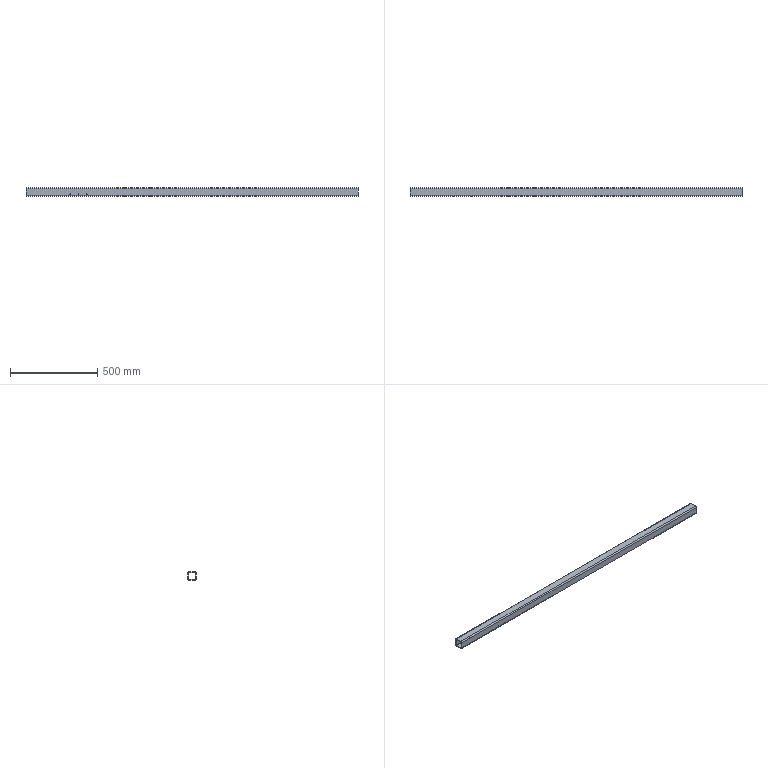Part | NX | 1 solid | 21 faces | box 1900 x 50 x 50 mm | volume 1636478 mm3 | cylinder 11 | plane 10 | commonest cylinder face diameters 4 x4 14 x4 3.3 x3
STEP:
#1=CARTESIAN_POINT('',(-950.,838.,555.));
#2=VERTEX_POINT('',#1);
#3=CARTESIAN_POINT('',(950.,838.,555.));
#4=VERTEX_POINT('',#3);
#5=CARTESIAN_POINT('',(-975.,838.,555.));
#6=DIRECTION('',(1.,0.,0.));
#7=VECTOR('',#6,1000.);
#8=LINE('',#5,#7);
#9=EDGE_CURVE('',#2,#4,#8,.T.);
#10=ORIENTED_EDGE('',*,*,#9,.T.);
#11=CARTESIAN_POINT('',(950.,874.,555.));
#12=VERTEX_POINT('',#11);
#13=CARTESIAN_POINT('',(950.,838.,555.));
#14=DIRECTION('',(0.,1.,0.));
#15=VECTOR('',#14,1000.);
#16=LINE('',#13,#15);
#17=EDGE_CURVE('',#4,#12,#16,.T.);
#18=ORIENTED_EDGE('',*,*,#17,.T.);
#19=CARTESIAN_POINT('',(-950.,874.,555.));
#20=VERTEX_POINT('',#19);
#21=CARTESIAN_POINT('',(-975.,874.,555.));
#22=DIRECTION('',(1.,0.,0.));
#23=VECTOR('',#22,1000.);
#24=LINE('',#21,#23);
#25=EDGE_CURVE('',#20,#12,#24,.T.);
#26=ORIENTED_EDGE('',*,*,#25,.F.);
#27=CARTESIAN_POINT('',(-950.,838.,555.));
#28=DIRECTION('',(0.,-1.,0.));
#29=VECTOR('',#28,1000.);
#30=LINE('',#27,#29);
#31=EDGE_CURVE('',#20,#2,#30,.T.);
#32=ORIENTED_EDGE('',*,*,#31,.T.);
#33=EDGE_LOOP('',(#10,#18,#26,#32));
#34=FACE_BOUND('',#33,.T.);
#35=CARTESIAN_POINT('',(-975.,838.,555.));
#36=DIRECTION('',(0.,0.,1.));
#37=DIRECTION('',(0.,-1.,0.));
#38=AXIS2_PLACEMENT_3D('',#35,#36,#37);
#39=PLANE('',#38);
#40=ADVANCED_FACE('',(#34),#39,.T.);
#41=CARTESIAN_POINT('',(-950.,836.,557.));
#42=VERTEX_POINT('',#41);
#43=CARTESIAN_POINT('',(950.,836.,557.));
#44=VERTEX_POINT('',#43);
#45=CARTESIAN_POINT('',(-975.,836.,557.));
#46=DIRECTION('',(1.,0.,0.));
#47=VECTOR('',#46,1000.);
#48=LINE('',#45,#47);
#49=EDGE_CURVE('',#42,#44,#48,.T.);
#50=ORIENTED_EDGE('',*,*,#49,.T.);
#51=CARTESIAN_POINT('',(950.,838.,557.));
#52=DIRECTION('',(1.,0.,0.));
#53=DIRECTION('',(0.,1.,0.));
#54=AXIS2_PLACEMENT_3D('',#51,#52,#53);
#55=CIRCLE('',#54,2.);
#56=EDGE_CURVE('',#44,#4,#55,.T.);
#57=ORIENTED_EDGE('',*,*,#56,.T.);
#58=ORIENTED_EDGE('',*,*,#9,.F.);
#59=CARTESIAN_POINT('',(-950.,838.,557.));
#60=DIRECTION('',(-1.,0.,0.));
#61=DIRECTION('',(0.,-1.,0.));
#62=AXIS2_PLACEMENT_3D('',#59,#60,#61);
#63=CIRCLE('',#62,2.);
#64=EDGE_CURVE('',#2,#42,#63,.T.);
#65=ORIENTED_EDGE('',*,*,#64,.T.);
#66=EDGE_LOOP('',(#50,#57,#58,#65));
#67=FACE_BOUND('',#66,.T.);
#68=CARTESIAN_POINT('',(-975.,838.,557.));
#69=DIRECTION('',(1.,0.,0.));
#70=DIRECTION('',(0.,0.,-1.));
#71=AXIS2_PLACEMENT_3D('',#68,#69,#70);
#72=CYLINDRICAL_SURFACE('',#71,2.);
#73=ADVANCED_FACE('',(#67),#72,.F.);
#74=CARTESIAN_POINT('',(-650.,836.,560.35));
#75=VERTEX_POINT('',#74);
#76=CARTESIAN_POINT('',(-650.,836.,562.));
#77=DIRECTION('',(0.,-1.,0.));
#78=DIRECTION('',(0.,0.,-1.));
#79=AXIS2_PLACEMENT_3D('',#76,#77,#78);
#80=CIRCLE('',#79,1.65);
#81=EDGE_CURVE('',#75,#75,#80,.T.);
#82=ORIENTED_EDGE('',*,*,#81,.T.);
#83=EDGE_LOOP('',(#82));
#84=FACE_BOUND('',#83,.T.);
#85=CARTESIAN_POINT('',(-602.5,836.,560.35));
#86=VERTEX_POINT('',#85);
#87=CARTESIAN_POINT('',(-602.5,836.,562.));
#88=DIRECTION('',(0.,-1.,0.));
#89=DIRECTION('',(0.,0.,-1.));
#90=AXIS2_PLACEMENT_3D('',#87,#88,#89);
#91=CIRCLE('',#90,1.65);
#92=EDGE_CURVE('',#86,#86,#91,.T.);
#93=ORIENTED_EDGE('',*,*,#92,.T.);
#94=EDGE_LOOP('',(#93));
#95=FACE_BOUND('',#94,.T.);
#96=CARTESIAN_POINT('',(-697.5,836.,560.35));
#97=VERTEX_POINT('',#96);
#98=CARTESIAN_POINT('',(-697.5,836.,562.));
#99=DIRECTION('',(0.,-1.,0.));
#100=DIRECTION('',(0.,0.,-1.));
#101=AXIS2_PLACEMENT_3D('',#98,#99,#100);
#102=CIRCLE('',#101,1.65);
#103=EDGE_CURVE('',#97,#97,#102,.T.);
#104=ORIENTED_EDGE('',*,*,#103,.T.);
#105=EDGE_LOOP('',(#104));
#106=FACE_BOUND('',#105,.T.);
#107=CARTESIAN_POINT('',(-950.,836.,593.));
#108=VERTEX_POINT('',#107);
#109=CARTESIAN_POINT('',(950.,836.,593.));
#110=VERTEX_POINT('',#109);
#111=CARTESIAN_POINT('',(-975.,836.,593.));
#112=DIRECTION('',(1.,0.,0.));
#113=VECTOR('',#112,1000.);
#114=LINE('',#111,#113);
#115=EDGE_CURVE('',#108,#110,#114,.T.);
#116=ORIENTED_EDGE('',*,*,#115,.T.);
#117=CARTESIAN_POINT('',(950.,836.,557.));
#118=DIRECTION('',(0.,0.,-1.));
#119=VECTOR('',#118,1000.);
#120=LINE('',#117,#119);
#121=EDGE_CURVE('',#110,#44,#120,.T.);
#122=ORIENTED_EDGE('',*,*,#121,.T.);
#123=ORIENTED_EDGE('',*,*,#49,.F.);
#124=CARTESIAN_POINT('',(-950.,836.,557.));
#125=DIRECTION('',(0.,0.,1.));
#126=VECTOR('',#125,1000.);
#127=LINE('',#124,#126);
#128=EDGE_CURVE('',#42,#108,#127,.T.);
#129=ORIENTED_EDGE('',*,*,#128,.T.);
#130=EDGE_LOOP('',(#116,#122,#123,#129));
#131=FACE_BOUND('',#130,.T.);
#132=CARTESIAN_POINT('',(-975.,836.,557.));
#133=DIRECTION('',(0.,1.,0.));
#134=DIRECTION('',(0.,0.,1.));
#135=AXIS2_PLACEMENT_3D('',#132,#133,#134);
#136=PLANE('',#135);
#137=ADVANCED_FACE('',(#84,#95,#106,#131),#136,.T.);
#138=CARTESIAN_POINT('',(-950.,838.,595.));
#139=VERTEX_POINT('',#138);
#140=CARTESIAN_POINT('',(950.,838.,595.));
#141=VERTEX_POINT('',#140);
#142=CARTESIAN_POINT('',(-975.,838.,595.));
#143=DIRECTION('',(1.,0.,0.));
#144=VECTOR('',#143,1000.);
#145=LINE('',#142,#144);
#146=EDGE_CURVE('',#139,#141,#145,.T.);
#147=ORIENTED_EDGE('',*,*,#146,.T.);
#148=CARTESIAN_POINT('',(950.,838.,593.));
#149=DIRECTION('',(1.,0.,0.));
#150=DIRECTION('',(0.,1.,0.));
#151=AXIS2_PLACEMENT_3D('',#148,#149,#150);
#152=CIRCLE('',#151,2.);
#153=EDGE_CURVE('',#141,#110,#152,.T.);
#154=ORIENTED_EDGE('',*,*,#153,.T.);
#155=ORIENTED_EDGE('',*,*,#115,.F.);
#156=CARTESIAN_POINT('',(-950.,838.,593.));
#157=DIRECTION('',(-1.,0.,0.));
#158=DIRECTION('',(0.,-1.,0.));
#159=AXIS2_PLACEMENT_3D('',#156,#157,#158);
#160=CIRCLE('',#159,2.);
#161=EDGE_CURVE('',#108,#139,#160,.T.);
#162=ORIENTED_EDGE('',*,*,#161,.T.);
#163=EDGE_LOOP('',(#147,#154,#155,#162));
#164=FACE_BOUND('',#163,.T.);
#165=CARTESIAN_POINT('',(-975.,838.,593.));
#166=DIRECTION('',(1.,0.,0.));
#167=DIRECTION('',(0.,0.,-1.));
#168=AXIS2_PLACEMENT_3D('',#165,#166,#167);
#169=CYLINDRICAL_SURFACE('',#168,2.);
#170=ADVANCED_FACE('',(#164),#169,.F.);
#171=CARTESIAN_POINT('',(-950.,874.,595.));
#172=VERTEX_POINT('',#171);
#173=CARTESIAN_POINT('',(950.,874.,595.));
#174=VERTEX_POINT('',#173);
#175=CARTESIAN_POINT('',(-975.,874.,595.));
#176=DIRECTION('',(1.,0.,0.));
#177=VECTOR('',#176,1000.);
#178=LINE('',#175,#177);
#179=EDGE_CURVE('',#172,#174,#178,.T.);
#180=ORIENTED_EDGE('',*,*,#179,.T.);
#181=CARTESIAN_POINT('',(950.,874.,595.));
#182=DIRECTION('',(0.,-1.,0.));
#183=VECTOR('',#182,1000.);
#184=LINE('',#181,#183);
#185=EDGE_CURVE('',#174,#141,#184,.T.);
#186=ORIENTED_EDGE('',*,*,#185,.T.);
#187=ORIENTED_EDGE('',*,*,#146,.F.);
#188=CARTESIAN_POINT('',(-950.,874.,595.));
#189=DIRECTION('',(0.,1.,0.));
#190=VECTOR('',#189,1000.);
#191=LINE('',#188,#190);
#192=EDGE_CURVE('',#139,#172,#191,.T.);
#193=ORIENTED_EDGE('',*,*,#192,.T.);
#194=EDGE_LOOP('',(#180,#186,#187,#193));
#195=FACE_BOUND('',#194,.T.);
#196=CARTESIAN_POINT('',(-975.,874.,595.));
#197=DIRECTION('',(0.,0.,-1.));
#198=DIRECTION('',(0.,1.,0.));
#199=AXIS2_PLACEMENT_3D('',#196,#197,#198);
#200=PLANE('',#199);
#201=ADVANCED_FACE('',(#195),#200,.T.);
#202=CARTESIAN_POINT('',(-950.,876.,593.));
#203=VERTEX_POINT('',#202);
#204=CARTESIAN_POINT('',(950.,876.,593.));
#205=VERTEX_POINT('',#204);
#206=CARTESIAN_POINT('',(-975.,876.,593.));
#207=DIRECTION('',(1.,0.,0.));
#208=VECTOR('',#207,1000.);
#209=LINE('',#206,#208);
#210=EDGE_CURVE('',#203,#205,#209,.T.);
#211=ORIENTED_EDGE('',*,*,#210,.T.);
#212=CARTESIAN_POINT('',(950.,874.,593.));
#213=DIRECTION('',(1.,0.,0.));
#214=DIRECTION('',(0.,1.,0.));
#215=AXIS2_PLACEMENT_3D('',#212,#213,#214);
#216=CIRCLE('',#215,2.);
#217=EDGE_CURVE('',#205,#174,#216,.T.);
#218=ORIENTED_EDGE('',*,*,#217,.T.);
#219=ORIENTED_EDGE('',*,*,#179,.F.);
#220=CARTESIAN_POINT('',(-950.,874.,593.));
#221=DIRECTION('',(-1.,0.,0.));
#222=DIRECTION('',(0.,-1.,0.));
#223=AXIS2_PLACEMENT_3D('',#220,#221,#222);
#224=CIRCLE('',#223,2.);
#225=EDGE_CURVE('',#172,#203,#224,.T.);
#226=ORIENTED_EDGE('',*,*,#225,.T.);
#227=EDGE_LOOP('',(#211,#218,#219,#226));
#228=FACE_BOUND('',#227,.T.);
#229=CARTESIAN_POINT('',(-975.,874.,593.));
#230=DIRECTION('',(1.,0.,0.));
#231=DIRECTION('',(0.,0.,-1.));
#232=AXIS2_PLACEMENT_3D('',#229,#230,#231);
#233=CYLINDRICAL_SURFACE('',#232,2.);
#234=ADVANCED_FACE('',(#228),#233,.F.);
#235=CARTESIAN_POINT('',(-950.,876.,557.));
#236=VERTEX_POINT('',#235);
#237=CARTESIAN_POINT('',(950.,876.,557.));
#238=VERTEX_POINT('',#237);
#239=CARTESIAN_POINT('',(-975.,876.,557.));
#240=DIRECTION('',(1.,0.,0.));
#241=VECTOR('',#240,1000.);
#242=LINE('',#239,#241);
#243=EDGE_CURVE('',#236,#238,#242,.T.);
#244=ORIENTED_EDGE('',*,*,#243,.T.);
#245=CARTESIAN_POINT('',(950.,876.,593.));
#246=DIRECTION('',(0.,0.,1.));
#247=VECTOR('',#246,1000.);
#248=LINE('',#245,#247);
#249=EDGE_CURVE('',#238,#205,#248,.T.);
#250=ORIENTED_EDGE('',*,*,#249,.T.);
#251=ORIENTED_EDGE('',*,*,#210,.F.);
#252=CARTESIAN_POINT('',(-950.,876.,593.));
#253=DIRECTION('',(0.,0.,-1.));
#254=VECTOR('',#253,1000.);
#255=LINE('',#252,#254);
#256=EDGE_CURVE('',#203,#236,#255,.T.);
#257=ORIENTED_EDGE('',*,*,#256,.T.);
#258=EDGE_LOOP('',(#244,#250,#251,#257));
#259=FACE_BOUND('',#258,.T.);
#260=CARTESIAN_POINT('',(-975.,876.,593.));
#261=DIRECTION('',(0.,-1.,0.));
#262=DIRECTION('',(0.,0.,-1.));
#263=AXIS2_PLACEMENT_3D('',#260,#261,#262);
#264=PLANE('',#263);
#265=ADVANCED_FACE('',(#259),#264,.T.);
#266=ORIENTED_EDGE('',*,*,#25,.T.);
#267=CARTESIAN_POINT('',(950.,874.,557.));
#268=DIRECTION('',(1.,0.,0.));
#269=DIRECTION('',(0.,1.,0.));
#270=AXIS2_PLACEMENT_3D('',#267,#268,#269);
#271=CIRCLE('',#270,2.);
#272=EDGE_CURVE('',#12,#238,#271,.T.);
#273=ORIENTED_EDGE('',*,*,#272,.T.);
#274=ORIENTED_EDGE('',*,*,#243,.F.);
#275=CARTESIAN_POINT('',(-950.,874.,557.));
#276=DIRECTION('',(-1.,0.,0.));
#277=DIRECTION('',(0.,-1.,0.));
#278=AXIS2_PLACEMENT_3D('',#275,#276,#277);
#279=CIRCLE('',#278,2.);
#280=EDGE_CURVE('',#236,#20,#279,.T.);
#281=ORIENTED_EDGE('',*,*,#280,.T.);
#282=EDGE_LOOP('',(#266,#273,#274,#281));
#283=FACE_BOUND('',#282,.T.);
#284=CARTESIAN_POINT('',(-975.,874.,557.));
#285=DIRECTION('',(1.,0.,0.));
#286=DIRECTION('',(0.,0.,-1.));
#287=AXIS2_PLACEMENT_3D('',#284,#285,#286);
#288=CYLINDRICAL_SURFACE('',#287,2.);
#289=ADVANCED_FACE('',(#283),#288,.F.);
#290=ORIENTED_EDGE('',*,*,#256,.F.);
#291=ORIENTED_EDGE('',*,*,#225,.F.);
#292=ORIENTED_EDGE('',*,*,#192,.F.);
#293=ORIENTED_EDGE('',*,*,#161,.F.);
#294=ORIENTED_EDGE('',*,*,#128,.F.);
#295=ORIENTED_EDGE('',*,*,#64,.F.);
#296=ORIENTED_EDGE('',*,*,#31,.F.);
#297=ORIENTED_EDGE('',*,*,#280,.F.);
#298=EDGE_LOOP('',(#290,#291,#292,#293,#294,#295,#296,#297));
#299=FACE_BOUND('',#298,.T.);
#300=CARTESIAN_POINT('',(-950.,874.,600.));
#301=VERTEX_POINT('',#300);
#302=CARTESIAN_POINT('',(-950.,881.,593.));
#303=VERTEX_POINT('',#302);
#304=CARTESIAN_POINT('',(-950.,874.,593.));
#305=DIRECTION('',(-1.,0.,0.));
#306=DIRECTION('',(0.,-1.,0.));
#307=AXIS2_PLACEMENT_3D('',#304,#305,#306);
#308=CIRCLE('',#307,7.);
#309=EDGE_CURVE('',#301,#303,#308,.T.);
#310=ORIENTED_EDGE('',*,*,#309,.T.);
#311=CARTESIAN_POINT('',(-950.,881.,557.));
#312=VERTEX_POINT('',#311);
#313=CARTESIAN_POINT('',(-950.,881.,593.));
#314=DIRECTION('',(0.,0.,-1.));
#315=VECTOR('',#314,1000.);
#316=LINE('',#313,#315);
#317=EDGE_CURVE('',#303,#312,#316,.T.);
#318=ORIENTED_EDGE('',*,*,#317,.T.);
#319=CARTESIAN_POINT('',(-950.,874.,550.));
#320=VERTEX_POINT('',#319);
#321=CARTESIAN_POINT('',(-950.,874.,557.));
#322=DIRECTION('',(-1.,0.,0.));
#323=DIRECTION('',(0.,-1.,0.));
#324=AXIS2_PLACEMENT_3D('',#321,#322,#323);
#325=CIRCLE('',#324,7.);
#326=EDGE_CURVE('',#312,#320,#325,.T.);
#327=ORIENTED_EDGE('',*,*,#326,.T.);
#328=CARTESIAN_POINT('',(-950.,838.,550.));
#329=VERTEX_POINT('',#328);
#330=CARTESIAN_POINT('',(-950.,0.,550.));
#331=DIRECTION('',(0.,1.,0.));
#332=VECTOR('',#331,1000.);
#333=LINE('',#330,#332);
#334=EDGE_CURVE('',#329,#320,#333,.T.);
#335=ORIENTED_EDGE('',*,*,#334,.F.);
#336=CARTESIAN_POINT('',(-950.,831.,557.));
#337=VERTEX_POINT('',#336);
#338=CARTESIAN_POINT('',(-950.,838.,557.));
#339=DIRECTION('',(-1.,0.,0.));
#340=DIRECTION('',(0.,-1.,0.));
#341=AXIS2_PLACEMENT_3D('',#338,#339,#340);
#342=CIRCLE('',#341,7.);
#343=EDGE_CURVE('',#329,#337,#342,.T.);
#344=ORIENTED_EDGE('',*,*,#343,.T.);
#345=CARTESIAN_POINT('',(-950.,831.,593.));
#346=VERTEX_POINT('',#345);
#347=CARTESIAN_POINT('',(-950.,831.,557.));
#348=DIRECTION('',(0.,0.,1.));
#349=VECTOR('',#348,1000.);
#350=LINE('',#347,#349);
#351=EDGE_CURVE('',#337,#346,#350,.T.);
#352=ORIENTED_EDGE('',*,*,#351,.T.);
#353=CARTESIAN_POINT('',(-950.,838.,600.));
#354=VERTEX_POINT('',#353);
#355=CARTESIAN_POINT('',(-950.,838.,593.));
#356=DIRECTION('',(-1.,0.,0.));
#357=DIRECTION('',(0.,-1.,0.));
#358=AXIS2_PLACEMENT_3D('',#355,#356,#357);
#359=CIRCLE('',#358,7.);
#360=EDGE_CURVE('',#346,#354,#359,.T.);
#361=ORIENTED_EDGE('',*,*,#360,.T.);
#362=CARTESIAN_POINT('',(-950.,874.,600.));
#363=DIRECTION('',(0.,1.,0.));
#364=VECTOR('',#363,1000.);
#365=LINE('',#362,#364);
#366=EDGE_CURVE('',#354,#301,#365,.T.);
#367=ORIENTED_EDGE('',*,*,#366,.T.);
#368=EDGE_LOOP('',(#310,#318,#327,#335,#344,#352,#361,#367));
#369=FACE_BOUND('',#368,.T.);
#370=CARTESIAN_POINT('',(-950.,0.,593.));
#371=DIRECTION('',(-1.,0.,0.));
#372=DIRECTION('',(0.,-1.,0.));
#373=AXIS2_PLACEMENT_3D('',#370,#371,#372);
#374=PLANE('',#373);
#375=ADVANCED_FACE('',(#299,#369),#374,.T.);
#376=CARTESIAN_POINT('',(950.,874.,600.));
#377=VERTEX_POINT('',#376);
#378=CARTESIAN_POINT('',(950.,838.,600.));
#379=VERTEX_POINT('',#378);
#380=CARTESIAN_POINT('',(950.,874.,600.));
#381=DIRECTION('',(0.,-1.,0.));
#382=VECTOR('',#381,1000.);
#383=LINE('',#380,#382);
#384=EDGE_CURVE('',#377,#379,#383,.T.);
#385=ORIENTED_EDGE('',*,*,#384,.F.);
#386=CARTESIAN_POINT('',(-975.,874.,600.));
#387=DIRECTION('',(1.,0.,0.));
#388=VECTOR('',#387,1000.);
#389=LINE('',#386,#388);
#390=EDGE_CURVE('',#301,#377,#389,.T.);
#391=ORIENTED_EDGE('',*,*,#390,.F.);
#392=ORIENTED_EDGE('',*,*,#366,.F.);
#393=CARTESIAN_POINT('',(-975.,838.,600.));
#394=DIRECTION('',(1.,0.,0.));
#395=VECTOR('',#394,1000.);
#396=LINE('',#393,#395);
#397=EDGE_CURVE('',#354,#379,#396,.T.);
#398=ORIENTED_EDGE('',*,*,#397,.T.);
#399=EDGE_LOOP('',(#385,#391,#392,#398));
#400=FACE_BOUND('',#399,.T.);
#401=CARTESIAN_POINT('',(-975.,874.,600.));
#402=DIRECTION('',(0.,0.,-1.));
#403=DIRECTION('',(0.,1.,0.));
#404=AXIS2_PLACEMENT_3D('',#401,#402,#403);
#405=PLANE('',#404);
#406=ADVANCED_FACE('',(#400),#405,.F.);
#407=CARTESIAN_POINT('',(950.,831.,593.));
#408=VERTEX_POINT('',#407);
#409=CARTESIAN_POINT('',(950.,838.,593.));
#410=DIRECTION('',(1.,0.,0.));
#411=DIRECTION('',(0.,1.,0.));
#412=AXIS2_PLACEMENT_3D('',#409,#410,#411);
#413=CIRCLE('',#412,7.);
#414=EDGE_CURVE('',#379,#408,#413,.T.);
#415=ORIENTED_EDGE('',*,*,#414,.F.);
#416=ORIENTED_EDGE('',*,*,#397,.F.);
#417=ORIENTED_EDGE('',*,*,#360,.F.);
#418=CARTESIAN_POINT('',(-975.,831.,593.));
#419=DIRECTION('',(1.,0.,0.));
#420=VECTOR('',#419,1000.);
#421=LINE('',#418,#420);
#422=EDGE_CURVE('',#346,#408,#421,.T.);
#423=ORIENTED_EDGE('',*,*,#422,.T.);
#424=EDGE_LOOP('',(#415,#416,#417,#423));
#425=FACE_BOUND('',#424,.T.);
#426=CARTESIAN_POINT('',(-975.,838.,593.));
#427=DIRECTION('',(1.,0.,0.));
#428=DIRECTION('',(0.,0.,-1.));
#429=AXIS2_PLACEMENT_3D('',#426,#427,#428);
#430=CYLINDRICAL_SURFACE('',#429,7.);
#431=ADVANCED_FACE('',(#425),#430,.T.);
#432=CARTESIAN_POINT('',(-650.,831.,563.65));
#433=VERTEX_POINT('',#432);
#434=CARTESIAN_POINT('',(-650.,831.,562.));
#435=DIRECTION('',(0.,1.,0.));
#436=DIRECTION('',(0.,0.,1.));
#437=AXIS2_PLACEMENT_3D('',#434,#435,#436);
#438=CIRCLE('',#437,1.65);
#439=EDGE_CURVE('',#433,#433,#438,.T.);
#440=ORIENTED_EDGE('',*,*,#439,.T.);
#441=EDGE_LOOP('',(#440));
#442=FACE_BOUND('',#441,.T.);
#443=CARTESIAN_POINT('',(-602.5,831.,563.65));
#444=VERTEX_POINT('',#443);
#445=CARTESIAN_POINT('',(-602.5,831.,562.));
#446=DIRECTION('',(0.,1.,0.));
#447=DIRECTION('',(0.,0.,1.));
#448=AXIS2_PLACEMENT_3D('',#445,#446,#447);
#449=CIRCLE('',#448,1.65);
#450=EDGE_CURVE('',#444,#444,#449,.T.);
#451=ORIENTED_EDGE('',*,*,#450,.T.);
#452=EDGE_LOOP('',(#451));
#453=FACE_BOUND('',#452,.T.);
#454=CARTESIAN_POINT('',(-697.5,831.,563.65));
#455=VERTEX_POINT('',#454);
#456=CARTESIAN_POINT('',(-697.5,831.,562.));
#457=DIRECTION('',(0.,1.,0.));
#458=DIRECTION('',(0.,0.,1.));
#459=AXIS2_PLACEMENT_3D('',#456,#457,#458);
#460=CIRCLE('',#459,1.65);
#461=EDGE_CURVE('',#455,#455,#460,.T.);
#462=ORIENTED_EDGE('',*,*,#461,.T.);
#463=EDGE_LOOP('',(#462));
#464=FACE_BOUND('',#463,.T.);
#465=CARTESIAN_POINT('',(950.,831.,557.));
#466=VERTEX_POINT('',#465);
#467=CARTESIAN_POINT('',(950.,831.,557.));
#468=DIRECTION('',(0.,0.,-1.));
#469=VECTOR('',#468,1000.);
#470=LINE('',#467,#469);
#471=EDGE_CURVE('',#408,#466,#470,.T.);
#472=ORIENTED_EDGE('',*,*,#471,.F.);
#473=ORIENTED_EDGE('',*,*,#422,.F.);
#474=ORIENTED_EDGE('',*,*,#351,.F.);
#475=CARTESIAN_POINT('',(-975.,831.,557.));
#476=DIRECTION('',(1.,0.,0.));
#477=VECTOR('',#476,1000.);
#478=LINE('',#475,#477);
#479=EDGE_CURVE('',#337,#466,#478,.T.);
#480=ORIENTED_EDGE('',*,*,#479,.T.);
#481=EDGE_LOOP('',(#472,#473,#474,#480));
#482=FACE_BOUND('',#481,.T.);
#483=CARTESIAN_POINT('',(-975.,831.,557.));
#484=DIRECTION('',(0.,1.,0.));
#485=DIRECTION('',(0.,0.,1.));
#486=AXIS2_PLACEMENT_3D('',#483,#484,#485);
#487=PLANE('',#486);
#488=ADVANCED_FACE('',(#442,#453,#464,#482),#487,.F.);
#489=CARTESIAN_POINT('',(950.,838.,550.));
#490=VERTEX_POINT('',#489);
#491=CARTESIAN_POINT('',(950.,838.,557.));
#492=DIRECTION('',(1.,0.,0.));
#493=DIRECTION('',(0.,1.,0.));
#494=AXIS2_PLACEMENT_3D('',#491,#492,#493);
#495=CIRCLE('',#494,7.);
#496=EDGE_CURVE('',#466,#490,#495,.T.);
#497=ORIENTED_EDGE('',*,*,#496,.F.);
#498=ORIENTED_EDGE('',*,*,#479,.F.);
#499=ORIENTED_EDGE('',*,*,#343,.F.);
#500=CARTESIAN_POINT('',(-975.,838.,550.));
#501=DIRECTION('',(1.,0.,0.));
#502=VECTOR('',#501,1000.);
#503=LINE('',#500,#502);
#504=EDGE_CURVE('',#329,#490,#503,.T.);
#505=ORIENTED_EDGE('',*,*,#504,.T.);
#506=EDGE_LOOP('',(#497,#498,#499,#505));
#507=FACE_BOUND('',#506,.T.);
#508=CARTESIAN_POINT('',(-975.,838.,557.));
#509=DIRECTION('',(1.,0.,0.));
#510=DIRECTION('',(0.,0.,-1.));
#511=AXIS2_PLACEMENT_3D('',#508,#509,#510);
#512=CYLINDRICAL_SURFACE('',#511,7.);
#513=ADVANCED_FACE('',(#507),#512,.T.);
#514=CARTESIAN_POINT('',(950.,874.,550.));
#515=VERTEX_POINT('',#514);
#516=CARTESIAN_POINT('',(950.,0.,550.));
#517=DIRECTION('',(0.,1.,0.));
#518=VECTOR('',#517,1000.);
#519=LINE('',#516,#518);
#520=EDGE_CURVE('',#490,#515,#519,.T.);
#521=ORIENTED_EDGE('',*,*,#520,.F.);
#522=ORIENTED_EDGE('',*,*,#504,.F.);
#523=ORIENTED_EDGE('',*,*,#334,.T.);
#524=CARTESIAN_POINT('',(-975.,874.,550.));
#525=DIRECTION('',(1.,0.,0.));
#526=VECTOR('',#525,1000.);
#527=LINE('',#524,#526);
#528=EDGE_CURVE('',#320,#515,#527,.T.);
#529=ORIENTED_EDGE('',*,*,#528,.T.);
#530=EDGE_LOOP('',(#521,#522,#523,#529));
#531=FACE_BOUND('',#530,.T.);
#532=CARTESIAN_POINT('',(-975.,838.,550.));
#533=DIRECTION('',(0.,0.,1.));
#534=DIRECTION('',(0.,-1.,0.));
#535=AXIS2_PLACEMENT_3D('',#532,#533,#534);
#536=PLANE('',#535);
#537=ADVANCED_FACE('',(#531),#536,.F.);
#538=CARTESIAN_POINT('',(950.,881.,557.));
#539=VERTEX_POINT('',#538);
#540=CARTESIAN_POINT('',(950.,874.,557.));
#541=DIRECTION('',(1.,0.,0.));
#542=DIRECTION('',(0.,1.,0.));
#543=AXIS2_PLACEMENT_3D('',#540,#541,#542);
#544=CIRCLE('',#543,7.);
#545=EDGE_CURVE('',#515,#539,#544,.T.);
#546=ORIENTED_EDGE('',*,*,#545,.F.);
#547=ORIENTED_EDGE('',*,*,#528,.F.);
#548=ORIENTED_EDGE('',*,*,#326,.F.);
#549=CARTESIAN_POINT('',(-975.,881.,557.));
#550=DIRECTION('',(1.,0.,0.));
#551=VECTOR('',#550,1000.);
#552=LINE('',#549,#551);
#553=EDGE_CURVE('',#312,#539,#552,.T.);
#554=ORIENTED_EDGE('',*,*,#553,.T.);
#555=EDGE_LOOP('',(#546,#547,#548,#554));
#556=FACE_BOUND('',#555,.T.);
#557=CARTESIAN_POINT('',(-975.,874.,557.));
#558=DIRECTION('',(1.,0.,0.));
#559=DIRECTION('',(0.,0.,-1.));
#560=AXIS2_PLACEMENT_3D('',#557,#558,#559);
#561=CYLINDRICAL_SURFACE('',#560,7.);
#562=ADVANCED_FACE('',(#556),#561,.T.);
#563=CARTESIAN_POINT('',(950.,881.,593.));
#564=VERTEX_POINT('',#563);
#565=CARTESIAN_POINT('',(950.,881.,593.));
#566=DIRECTION('',(0.,0.,1.));
#567=VECTOR('',#566,1000.);
#568=LINE('',#565,#567);
#569=EDGE_CURVE('',#539,#564,#568,.T.);
#570=ORIENTED_EDGE('',*,*,#569,.F.);
#571=ORIENTED_EDGE('',*,*,#553,.F.);
#572=ORIENTED_EDGE('',*,*,#317,.F.);
#573=CARTESIAN_POINT('',(-975.,881.,593.));
#574=DIRECTION('',(1.,0.,0.));
#575=VECTOR('',#574,1000.);
#576=LINE('',#573,#575);
#577=EDGE_CURVE('',#303,#564,#576,.T.);
#578=ORIENTED_EDGE('',*,*,#577,.T.);
#579=EDGE_LOOP('',(#570,#571,#572,#578));
#580=FACE_BOUND('',#579,.T.);
#581=CARTESIAN_POINT('',(-975.,881.,593.));
#582=DIRECTION('',(0.,-1.,0.));
#583=DIRECTION('',(0.,0.,-1.));
#584=AXIS2_PLACEMENT_3D('',#581,#582,#583);
#585=PLANE('',#584);
#586=ADVANCED_FACE('',(#580),#585,.F.);
#587=CARTESIAN_POINT('',(950.,874.,593.));
#588=DIRECTION('',(1.,0.,0.));
#589=DIRECTION('',(0.,1.,0.));
#590=AXIS2_PLACEMENT_3D('',#587,#588,#589);
#591=CIRCLE('',#590,7.);
#592=EDGE_CURVE('',#564,#377,#591,.T.);
#593=ORIENTED_EDGE('',*,*,#592,.F.);
#594=ORIENTED_EDGE('',*,*,#577,.F.);
#595=ORIENTED_EDGE('',*,*,#309,.F.);
#596=ORIENTED_EDGE('',*,*,#390,.T.);
#597=EDGE_LOOP('',(#593,#594,#595,#596));
#598=FACE_BOUND('',#597,.T.);
#599=CARTESIAN_POINT('',(-975.,874.,593.));
#600=DIRECTION('',(1.,0.,0.));
#601=DIRECTION('',(0.,0.,-1.));
#602=AXIS2_PLACEMENT_3D('',#599,#600,#601);
#603=CYLINDRICAL_SURFACE('',#602,7.);
#604=ADVANCED_FACE('',(#598),#603,.T.);
#605=ORIENTED_EDGE('',*,*,#17,.F.);
#606=ORIENTED_EDGE('',*,*,#56,.F.);
#607=ORIENTED_EDGE('',*,*,#121,.F.);
#608=ORIENTED_EDGE('',*,*,#153,.F.);
#609=ORIENTED_EDGE('',*,*,#185,.F.);
#610=ORIENTED_EDGE('',*,*,#217,.F.);
#611=ORIENTED_EDGE('',*,*,#249,.F.);
#612=ORIENTED_EDGE('',*,*,#272,.F.);
#613=EDGE_LOOP('',(#605,#606,#607,#608,#609,#610,#611,#612));
#614=FACE_BOUND('',#613,.T.);
#615=ORIENTED_EDGE('',*,*,#592,.T.);
#616=ORIENTED_EDGE('',*,*,#384,.T.);
#617=ORIENTED_EDGE('',*,*,#414,.T.);
#618=ORIENTED_EDGE('',*,*,#471,.T.);
#619=ORIENTED_EDGE('',*,*,#496,.T.);
#620=ORIENTED_EDGE('',*,*,#520,.T.);
#621=ORIENTED_EDGE('',*,*,#545,.T.);
#622=ORIENTED_EDGE('',*,*,#569,.T.);
#623=EDGE_LOOP('',(#615,#616,#617,#618,#619,#620,#621,#622));
#624=FACE_BOUND('',#623,.T.);
#625=CARTESIAN_POINT('',(950.,0.,557.));
#626=DIRECTION('',(1.,0.,0.));
#627=DIRECTION('',(0.,1.,0.));
#628=AXIS2_PLACEMENT_3D('',#625,#626,#627);
#629=PLANE('',#628);
#630=ADVANCED_FACE('',(#614,#624),#629,.T.);
#631=ORIENTED_EDGE('',*,*,#103,.F.);
#632=EDGE_LOOP('',(#631));
#633=FACE_BOUND('',#632,.T.);
#634=ORIENTED_EDGE('',*,*,#461,.F.);
#635=EDGE_LOOP('',(#634));
#636=FACE_BOUND('',#635,.T.);
#637=CARTESIAN_POINT('',(-697.5,831.,562.));
#638=DIRECTION('',(0.,-1.,0.));
#639=DIRECTION('',(0.,0.,1.));
#640=AXIS2_PLACEMENT_3D('',#637,#638,#639);
#641=CYLINDRICAL_SURFACE('',#640,1.65);
#642=ADVANCED_FACE('',(#633,#636),#641,.F.);
#643=ORIENTED_EDGE('',*,*,#92,.F.);
#644=EDGE_LOOP('',(#643));
#645=FACE_BOUND('',#644,.T.);
#646=ORIENTED_EDGE('',*,*,#450,.F.);
#647=EDGE_LOOP('',(#646));
#648=FACE_BOUND('',#647,.T.);
#649=CARTESIAN_POINT('',(-602.5,831.,562.));
#650=DIRECTION('',(0.,-1.,0.));
#651=DIRECTION('',(0.,0.,1.));
#652=AXIS2_PLACEMENT_3D('',#649,#650,#651);
#653=CYLINDRICAL_SURFACE('',#652,1.65);
#654=ADVANCED_FACE('',(#645,#648),#653,.F.);
#655=ORIENTED_EDGE('',*,*,#81,.F.);
#656=EDGE_LOOP('',(#655));
#657=FACE_BOUND('',#656,.T.);
#658=ORIENTED_EDGE('',*,*,#439,.F.);
#659=EDGE_LOOP('',(#658));
#660=FACE_BOUND('',#659,.T.);
#661=CARTESIAN_POINT('',(-650.,831.,562.));
#662=DIRECTION('',(0.,-1.,0.));
#663=DIRECTION('',(0.,0.,1.));
#664=AXIS2_PLACEMENT_3D('',#661,#662,#663);
#665=CYLINDRICAL_SURFACE('',#664,1.65);
#666=ADVANCED_FACE('',(#657,#660),#665,.F.);
#667=CLOSED_SHELL('',(#40,#73,#137,#170,#201,#234,#265,#289,#375,#406,#431,#488,#513,#537,#562,#586,#604,#630,#642,#654,#666));
#668=MANIFOLD_SOLID_BREP('',#667);
#669=(LENGTH_UNIT()NAMED_UNIT(*)SI_UNIT(.MILLI.,.METRE.));
#670=UNCERTAINTY_MEASURE_WITH_UNIT(LENGTH_MEASURE(0.00001),#669,'','');
#671=(NAMED_UNIT(*)PLANE_ANGLE_UNIT()SI_UNIT($,.RADIAN.));
#672=(NAMED_UNIT(*)SI_UNIT($,.STERADIAN.)SOLID_ANGLE_UNIT());
#673=(GEOMETRIC_REPRESENTATION_CONTEXT(3)GLOBAL_UNCERTAINTY_ASSIGNED_CONTEXT((#670))GLOBAL_UNIT_ASSIGNED_CONTEXT((#669,#671,#672))REPRESENTATION_CONTEXT('',''));
#674=ADVANCED_BREP_SHAPE_REPRESENTATION('',(#668),#673);